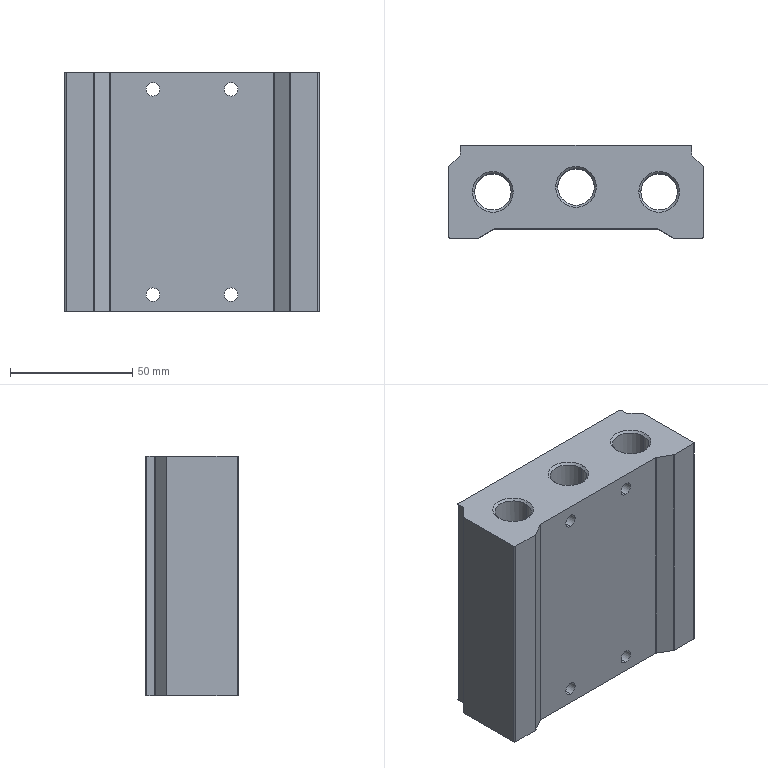Part | STEP file | 400M_2F_400M-2F | 1 solid | 94 faces | box 104 x 38 x 98 mm | volume 289660 mm3 | cylinder 44 | cone 28 | plane 22 | commonest cylinder face diameters 1 x10 3.242 x8 5.5 x8 12 x8 14.95 x6 14.5 x4